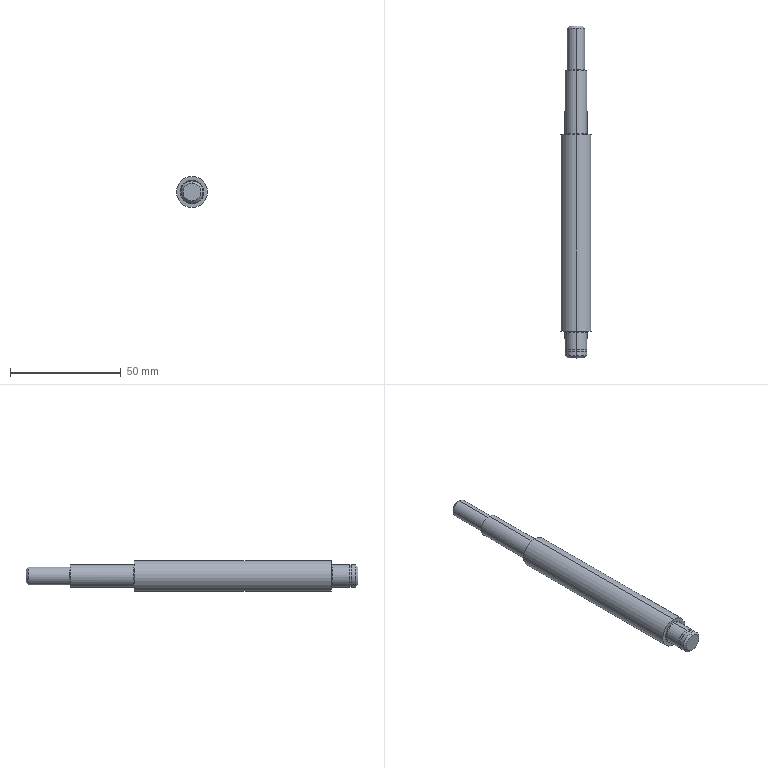Part | SolidWorks | features BaseBody 1 | 1 solid | 29 faces | box 14 x 150 x 14 mm | volume 17893 mm3 | cylinder 12 | plane 7 | spline 6 | cone 4 | commonest cylinder face diameters 10 x6 8 x2 9.6 x2 14 x2
STEP:
#1=CARTESIAN_POINT('',(295.521,1568.164,-1178.061));
#2=VERTEX_POINT('',#1);
#3=CARTESIAN_POINT('',(290.547,1568.164,-1173.57));
#4=VERTEX_POINT('',#3);
#5=CARTESIAN_POINT('',(290.547,1568.164,-1178.57));
#6=DIRECTION('',(0.,-1.,0.));
#7=DIRECTION('',(-0.9948,0.,-0.1018));
#8=AXIS2_PLACEMENT_3D('',#5,#6,#7);
#9=CIRCLE('',#8,5.);
#10=EDGE_CURVE('',#2,#4,#9,.T.);
#11=ORIENTED_EDGE('',*,*,#10,.F.);
#12=CARTESIAN_POINT('',(295.819,1568.464,-1178.031));
#13=VERTEX_POINT('',#12);
#14=CARTESIAN_POINT('',(295.819,1568.164,-1178.031));
#15=DIRECTION('',(0.1018,0.,-0.9948));
#16=DIRECTION('',(0.9948,0.,0.1018));
#17=AXIS2_PLACEMENT_3D('',#14,#15,#16);
#18=CIRCLE('',#17,0.3);
#19=EDGE_CURVE('',#2,#13,#18,.T.);
#20=ORIENTED_EDGE('',*,*,#19,.T.);
#21=CARTESIAN_POINT('',(285.274,1568.464,-1179.109));
#22=VERTEX_POINT('',#21);
#23=CARTESIAN_POINT('',(295.819,1568.464,-1178.031));
#24=CARTESIAN_POINT('',(295.503,1568.464,-1174.942));
#25=CARTESIAN_POINT('',(293.096,1568.464,-1172.982));
#26=CARTESIAN_POINT('',(290.007,1568.464,-1173.298));
#27=CARTESIAN_POINT('',(286.919,1568.464,-1173.613));
#28=CARTESIAN_POINT('',(284.958,1568.464,-1176.021));
#29=CARTESIAN_POINT('',(285.274,1568.464,-1179.109));
#30=(BOUNDED_CURVE()B_SPLINE_CURVE(3,(#23,#24,#25,#26,#27,#28,#29),.UNSPECIFIED.,.F.,.T.)B_SPLINE_CURVE_WITH_KNOTS((4,3,4),(0.,0.5,1.),.UNSPECIFIED.)CURVE()GEOMETRIC_REPRESENTATION_ITEM()RATIONAL_B_SPLINE_CURVE((1.,0.8047,0.8047,1.,0.8047,0.8047,1.))REPRESENTATION_ITEM(''));
#31=EDGE_CURVE('',#13,#22,#30,.T.);
#32=ORIENTED_EDGE('',*,*,#31,.T.);
#33=CARTESIAN_POINT('',(285.572,1568.164,-1179.079));
#34=VERTEX_POINT('',#33);
#35=CARTESIAN_POINT('',(285.274,1568.164,-1179.109));
#36=DIRECTION('',(-0.1018,0.,0.9948));
#37=DIRECTION('',(-0.9948,0.,-0.1018));
#38=AXIS2_PLACEMENT_3D('',#35,#36,#37);
#39=CIRCLE('',#38,0.3);
#40=EDGE_CURVE('',#34,#22,#39,.T.);
#41=ORIENTED_EDGE('',*,*,#40,.F.);
#42=CARTESIAN_POINT('',(290.547,1568.164,-1178.57));
#43=DIRECTION('',(0.,-1.,0.));
#44=DIRECTION('',(-0.9948,0.,-0.1018));
#45=AXIS2_PLACEMENT_3D('',#42,#43,#44);
#46=CIRCLE('',#45,5.);
#47=EDGE_CURVE('',#4,#34,#46,.T.);
#48=ORIENTED_EDGE('',*,*,#47,.F.);
#49=EDGE_LOOP('',(#11,#20,#32,#41,#48));
#50=FACE_OUTER_BOUND('',#49,.T.);
#51=CARTESIAN_POINT('',(285.572,1568.164,-1179.079));
#52=CARTESIAN_POINT('',(285.274,1568.164,-1176.165));
#53=CARTESIAN_POINT('',(287.124,1568.164,-1173.894));
#54=CARTESIAN_POINT('',(290.038,1568.164,-1173.596));
#55=CARTESIAN_POINT('',(292.951,1568.164,-1173.298));
#56=CARTESIAN_POINT('',(295.222,1568.164,-1175.147));
#57=CARTESIAN_POINT('',(295.521,1568.164,-1178.061));
#58=CARTESIAN_POINT('',(285.572,1568.34,-1179.079));
#59=CARTESIAN_POINT('',(285.274,1568.34,-1176.165));
#60=CARTESIAN_POINT('',(287.124,1568.34,-1173.894));
#61=CARTESIAN_POINT('',(290.038,1568.34,-1173.596));
#62=CARTESIAN_POINT('',(292.951,1568.34,-1173.298));
#63=CARTESIAN_POINT('',(295.222,1568.34,-1175.147));
#64=CARTESIAN_POINT('',(295.521,1568.34,-1178.061));
#65=CARTESIAN_POINT('',(285.449,1568.464,-1179.091));
#66=CARTESIAN_POINT('',(285.143,1568.464,-1176.105));
#67=CARTESIAN_POINT('',(287.039,1568.464,-1173.778));
#68=CARTESIAN_POINT('',(290.025,1568.464,-1173.472));
#69=CARTESIAN_POINT('',(293.011,1568.464,-1173.167));
#70=CARTESIAN_POINT('',(295.339,1568.464,-1175.062));
#71=CARTESIAN_POINT('',(295.644,1568.464,-1178.049));
#72=CARTESIAN_POINT('',(285.274,1568.464,-1179.109));
#73=CARTESIAN_POINT('',(284.958,1568.464,-1176.021));
#74=CARTESIAN_POINT('',(286.919,1568.464,-1173.613));
#75=CARTESIAN_POINT('',(290.007,1568.464,-1173.298));
#76=CARTESIAN_POINT('',(293.096,1568.464,-1172.982));
#77=CARTESIAN_POINT('',(295.503,1568.464,-1174.942));
#78=CARTESIAN_POINT('',(295.819,1568.464,-1178.031));
#79=(BOUNDED_SURFACE()B_SPLINE_SURFACE(3,3,((#51,#52,#53,#54,#55,#56,#57),(#58,#59,#60,#61,#62,#63,#64),(#65,#66,#67,#68,#69,#70,#71),(#72,#73,#74,#75,#76,#77,#78)),.UNSPECIFIED.,.F.,.F.,.F.)B_SPLINE_SURFACE_WITH_KNOTS((4,4),(4,3,4),(0.,1.),(0.,0.5,1.),.UNSPECIFIED.)GEOMETRIC_REPRESENTATION_ITEM()RATIONAL_B_SPLINE_SURFACE(((1.,0.8047,0.8047,1.,0.8047,0.8047,1.),(0.8047,0.6476,0.6476,0.8047,0.6476,0.6476,0.8047),(0.8047,0.6476,0.6476,0.8047,0.6476,0.6476,0.8047),(1.,0.8047,0.8047,1.,0.8047,0.8047,1.)))REPRESENTATION_ITEM('')SURFACE());
#80=ADVANCED_FACE('',(#50),#79,.F.);
#81=CARTESIAN_POINT('',(285.572,1657.764,-1179.079));
#82=VERTEX_POINT('',#81);
#83=CARTESIAN_POINT('',(290.547,1657.764,-1173.57));
#84=VERTEX_POINT('',#83);
#85=CARTESIAN_POINT('',(290.547,1657.764,-1178.57));
#86=DIRECTION('',(0.,1.,0.));
#87=DIRECTION('',(0.9948,0.,0.1018));
#88=AXIS2_PLACEMENT_3D('',#85,#86,#87);
#89=CIRCLE('',#88,5.);
#90=EDGE_CURVE('',#82,#84,#89,.T.);
#91=ORIENTED_EDGE('',*,*,#90,.F.);
#92=CARTESIAN_POINT('',(285.274,1657.464,-1179.109));
#93=VERTEX_POINT('',#92);
#94=CARTESIAN_POINT('',(285.274,1657.764,-1179.109));
#95=DIRECTION('',(0.1018,0.,-0.9948));
#96=DIRECTION('',(-0.9948,0.,-0.1018));
#97=AXIS2_PLACEMENT_3D('',#94,#95,#96);
#98=CIRCLE('',#97,0.3);
#99=EDGE_CURVE('',#82,#93,#98,.T.);
#100=ORIENTED_EDGE('',*,*,#99,.T.);
#101=CARTESIAN_POINT('',(295.819,1657.464,-1178.031));
#102=VERTEX_POINT('',#101);
#103=CARTESIAN_POINT('',(285.274,1657.464,-1179.109));
#104=CARTESIAN_POINT('',(284.958,1657.464,-1176.021));
#105=CARTESIAN_POINT('',(286.919,1657.464,-1173.613));
#106=CARTESIAN_POINT('',(290.007,1657.464,-1173.298));
#107=CARTESIAN_POINT('',(293.096,1657.464,-1172.982));
#108=CARTESIAN_POINT('',(295.503,1657.464,-1174.942));
#109=CARTESIAN_POINT('',(295.819,1657.464,-1178.031));
#110=(BOUNDED_CURVE()B_SPLINE_CURVE(3,(#103,#104,#105,#106,#107,#108,#109),.UNSPECIFIED.,.F.,.T.)B_SPLINE_CURVE_WITH_KNOTS((4,3,4),(0.,0.5,1.),.UNSPECIFIED.)CURVE()GEOMETRIC_REPRESENTATION_ITEM()RATIONAL_B_SPLINE_CURVE((1.,0.8047,0.8047,1.,0.8047,0.8047,1.))REPRESENTATION_ITEM(''));
#111=EDGE_CURVE('',#93,#102,#110,.T.);
#112=ORIENTED_EDGE('',*,*,#111,.T.);
#113=CARTESIAN_POINT('',(295.521,1657.764,-1178.061));
#114=VERTEX_POINT('',#113);
#115=CARTESIAN_POINT('',(295.819,1657.764,-1178.031));
#116=DIRECTION('',(-0.1018,0.,0.9948));
#117=DIRECTION('',(0.9948,0.,0.1018));
#118=AXIS2_PLACEMENT_3D('',#115,#116,#117);
#119=CIRCLE('',#118,0.3);
#120=EDGE_CURVE('',#114,#102,#119,.T.);
#121=ORIENTED_EDGE('',*,*,#120,.F.);
#122=CARTESIAN_POINT('',(290.547,1657.764,-1178.57));
#123=DIRECTION('',(0.,1.,0.));
#124=DIRECTION('',(0.9948,0.,0.1018));
#125=AXIS2_PLACEMENT_3D('',#122,#123,#124);
#126=CIRCLE('',#125,5.);
#127=EDGE_CURVE('',#84,#114,#126,.T.);
#128=ORIENTED_EDGE('',*,*,#127,.F.);
#129=EDGE_LOOP('',(#91,#100,#112,#121,#128));
#130=FACE_OUTER_BOUND('',#129,.T.);
#131=CARTESIAN_POINT('',(295.521,1657.764,-1178.061));
#132=CARTESIAN_POINT('',(295.222,1657.764,-1175.147));
#133=CARTESIAN_POINT('',(292.951,1657.764,-1173.298));
#134=CARTESIAN_POINT('',(290.038,1657.764,-1173.596));
#135=CARTESIAN_POINT('',(287.124,1657.764,-1173.894));
#136=CARTESIAN_POINT('',(285.274,1657.764,-1176.165));
#137=CARTESIAN_POINT('',(285.572,1657.764,-1179.079));
#138=CARTESIAN_POINT('',(295.521,1657.588,-1178.061));
#139=CARTESIAN_POINT('',(295.222,1657.588,-1175.147));
#140=CARTESIAN_POINT('',(292.951,1657.588,-1173.298));
#141=CARTESIAN_POINT('',(290.038,1657.588,-1173.596));
#142=CARTESIAN_POINT('',(287.124,1657.588,-1173.894));
#143=CARTESIAN_POINT('',(285.274,1657.588,-1176.165));
#144=CARTESIAN_POINT('',(285.572,1657.588,-1179.079));
#145=CARTESIAN_POINT('',(295.644,1657.464,-1178.049));
#146=CARTESIAN_POINT('',(295.339,1657.464,-1175.062));
#147=CARTESIAN_POINT('',(293.011,1657.464,-1173.167));
#148=CARTESIAN_POINT('',(290.025,1657.464,-1173.472));
#149=CARTESIAN_POINT('',(287.039,1657.464,-1173.778));
#150=CARTESIAN_POINT('',(285.143,1657.464,-1176.105));
#151=CARTESIAN_POINT('',(285.449,1657.464,-1179.091));
#152=CARTESIAN_POINT('',(295.819,1657.464,-1178.031));
#153=CARTESIAN_POINT('',(295.503,1657.464,-1174.942));
#154=CARTESIAN_POINT('',(293.096,1657.464,-1172.982));
#155=CARTESIAN_POINT('',(290.007,1657.464,-1173.298));
#156=CARTESIAN_POINT('',(286.919,1657.464,-1173.613));
#157=CARTESIAN_POINT('',(284.958,1657.464,-1176.021));
#158=CARTESIAN_POINT('',(285.274,1657.464,-1179.109));
#159=(BOUNDED_SURFACE()B_SPLINE_SURFACE(3,3,((#131,#132,#133,#134,#135,#136,#137),(#138,#139,#140,#141,#142,#143,#144),(#145,#146,#147,#148,#149,#150,#151),(#152,#153,#154,#155,#156,#157,#158)),.UNSPECIFIED.,.F.,.F.,.F.)B_SPLINE_SURFACE_WITH_KNOTS((4,4),(4,3,4),(0.,1.),(0.,0.5,1.),.UNSPECIFIED.)GEOMETRIC_REPRESENTATION_ITEM()RATIONAL_B_SPLINE_SURFACE(((1.,0.8047,0.8047,1.,0.8047,0.8047,1.),(0.8047,0.6476,0.6476,0.8047,0.6476,0.6476,0.8047),(0.8047,0.6476,0.6476,0.8047,0.6476,0.6476,0.8047),(1.,0.8047,0.8047,1.,0.8047,0.8047,1.)))REPRESENTATION_ITEM('')SURFACE());
#160=ADVANCED_FACE('',(#130),#159,.F.);
#161=CARTESIAN_POINT('',(286.567,1686.764,-1178.977));
#162=VERTEX_POINT('',#161);
#163=CARTESIAN_POINT('',(290.547,1686.764,-1174.57));
#164=VERTEX_POINT('',#163);
#165=CARTESIAN_POINT('',(290.547,1686.764,-1178.57));
#166=DIRECTION('',(0.,1.,0.));
#167=DIRECTION('',(0.9948,0.,0.1018));
#168=AXIS2_PLACEMENT_3D('',#165,#166,#167);
#169=CIRCLE('',#168,4.);
#170=EDGE_CURVE('',#162,#164,#169,.T.);
#171=ORIENTED_EDGE('',*,*,#170,.F.);
#172=CARTESIAN_POINT('',(286.269,1686.464,-1179.008));
#173=VERTEX_POINT('',#172);
#174=CARTESIAN_POINT('',(286.269,1686.764,-1179.008));
#175=DIRECTION('',(0.1018,0.,-0.9948));
#176=DIRECTION('',(-0.9948,0.,-0.1018));
#177=AXIS2_PLACEMENT_3D('',#174,#175,#176);
#178=CIRCLE('',#177,0.3);
#179=EDGE_CURVE('',#162,#173,#178,.T.);
#180=ORIENTED_EDGE('',*,*,#179,.T.);
#181=CARTESIAN_POINT('',(294.824,1686.464,-1178.132));
#182=VERTEX_POINT('',#181);
#183=CARTESIAN_POINT('',(286.269,1686.464,-1179.008));
#184=CARTESIAN_POINT('',(285.394,1686.464,-1170.452));
#185=CARTESIAN_POINT('',(293.949,1686.464,-1169.577));
#186=CARTESIAN_POINT('',(294.824,1686.464,-1178.132));
#187=(BOUNDED_CURVE()B_SPLINE_CURVE(3,(#183,#184,#185,#186),.UNSPECIFIED.,.F.,.T.)B_SPLINE_CURVE_WITH_KNOTS((4,4),(0.,1.),.UNSPECIFIED.)CURVE()GEOMETRIC_REPRESENTATION_ITEM()RATIONAL_B_SPLINE_CURVE((1.,0.3333,0.3333,1.))REPRESENTATION_ITEM(''));
#188=EDGE_CURVE('',#173,#182,#187,.T.);
#189=ORIENTED_EDGE('',*,*,#188,.T.);
#190=CARTESIAN_POINT('',(294.526,1686.764,-1178.163));
#191=VERTEX_POINT('',#190);
#192=CARTESIAN_POINT('',(294.824,1686.764,-1178.132));
#193=DIRECTION('',(-0.1018,0.,0.9948));
#194=DIRECTION('',(0.9948,0.,0.1018));
#195=AXIS2_PLACEMENT_3D('',#192,#193,#194);
#196=CIRCLE('',#195,0.3);
#197=EDGE_CURVE('',#191,#182,#196,.T.);
#198=ORIENTED_EDGE('',*,*,#197,.F.);
#199=CARTESIAN_POINT('',(290.547,1686.764,-1178.57));
#200=DIRECTION('',(0.,1.,0.));
#201=DIRECTION('',(0.9948,0.,0.1018));
#202=AXIS2_PLACEMENT_3D('',#199,#200,#201);
#203=CIRCLE('',#202,4.);
#204=EDGE_CURVE('',#164,#191,#203,.T.);
#205=ORIENTED_EDGE('',*,*,#204,.F.);
#206=EDGE_LOOP('',(#171,#180,#189,#198,#205));
#207=FACE_OUTER_BOUND('',#206,.T.);
#208=CARTESIAN_POINT('',(294.526,1686.764,-1178.163));
#209=CARTESIAN_POINT('',(293.712,1686.764,-1170.204));
#210=CARTESIAN_POINT('',(285.753,1686.764,-1171.019));
#211=CARTESIAN_POINT('',(286.567,1686.764,-1178.977));
#212=CARTESIAN_POINT('',(294.526,1686.588,-1178.163));
#213=CARTESIAN_POINT('',(293.712,1686.588,-1170.204));
#214=CARTESIAN_POINT('',(285.753,1686.588,-1171.019));
#215=CARTESIAN_POINT('',(286.567,1686.588,-1178.977));
#216=CARTESIAN_POINT('',(294.649,1686.464,-1178.15));
#217=CARTESIAN_POINT('',(293.81,1686.464,-1169.945));
#218=CARTESIAN_POINT('',(285.604,1686.464,-1170.784));
#219=CARTESIAN_POINT('',(286.444,1686.464,-1178.99));
#220=CARTESIAN_POINT('',(294.824,1686.464,-1178.132));
#221=CARTESIAN_POINT('',(293.949,1686.464,-1169.577));
#222=CARTESIAN_POINT('',(285.394,1686.464,-1170.452));
#223=CARTESIAN_POINT('',(286.269,1686.464,-1179.008));
#224=(BOUNDED_SURFACE()B_SPLINE_SURFACE(3,3,((#208,#209,#210,#211),(#212,#213,#214,#215),(#216,#217,#218,#219),(#220,#221,#222,#223)),.UNSPECIFIED.,.F.,.F.,.F.)B_SPLINE_SURFACE_WITH_KNOTS((4,4),(4,4),(0.,1.),(0.,1.),.UNSPECIFIED.)GEOMETRIC_REPRESENTATION_ITEM()RATIONAL_B_SPLINE_SURFACE(((1.,0.3333,0.3333,1.),(0.8047,0.2682,0.2682,0.8047),(0.8047,0.2682,0.2682,0.8047),(1.,0.3333,0.3333,1.)))REPRESENTATION_ITEM('')SURFACE());
#225=ADVANCED_FACE('',(#207),#224,.F.);
#226=CARTESIAN_POINT('',(290.547,1657.464,-1185.57));
#227=VERTEX_POINT('',#226);
#228=CARTESIAN_POINT('',(290.547,1657.464,-1171.57));
#229=VERTEX_POINT('',#228);
#230=CARTESIAN_POINT('',(290.547,1657.464,-1178.57));
#231=DIRECTION('',(0.,-1.,0.));
#232=DIRECTION('',(0.,0.,-1.));
#233=AXIS2_PLACEMENT_3D('',#230,#231,#232);
#234=CIRCLE('',#233,7.);
#235=EDGE_CURVE('',#227,#229,#234,.T.);
#236=ORIENTED_EDGE('',*,*,#235,.T.);
#237=CARTESIAN_POINT('',(290.547,1568.464,-1171.57));
#238=VERTEX_POINT('',#237);
#239=CARTESIAN_POINT('',(290.547,1556.464,-1171.57));
#240=DIRECTION('',(0.,-1.,0.));
#241=VECTOR('',#240,1000.);
#242=LINE('',#239,#241);
#243=EDGE_CURVE('',#229,#238,#242,.T.);
#244=ORIENTED_EDGE('',*,*,#243,.T.);
#245=CARTESIAN_POINT('',(290.547,1568.464,-1185.57));
#246=VERTEX_POINT('',#245);
#247=CARTESIAN_POINT('',(290.547,1568.464,-1178.57));
#248=DIRECTION('',(0.,1.,0.));
#249=DIRECTION('',(0.,0.,-1.));
#250=AXIS2_PLACEMENT_3D('',#247,#248,#249);
#251=CIRCLE('',#250,7.);
#252=EDGE_CURVE('',#238,#246,#251,.T.);
#253=ORIENTED_EDGE('',*,*,#252,.T.);
#254=CARTESIAN_POINT('',(290.547,1556.464,-1185.57));
#255=DIRECTION('',(0.,-1.,0.));
#256=VECTOR('',#255,1000.);
#257=LINE('',#254,#256);
#258=EDGE_CURVE('',#227,#246,#257,.T.);
#259=ORIENTED_EDGE('',*,*,#258,.F.);
#260=EDGE_LOOP('',(#236,#244,#253,#259));
#261=FACE_OUTER_BOUND('',#260,.T.);
#262=CARTESIAN_POINT('',(290.547,1556.464,-1178.57));
#263=DIRECTION('',(0.,-1.,0.));
#264=DIRECTION('',(0.,0.,-1.));
#265=AXIS2_PLACEMENT_3D('',#262,#263,#264);
#266=CYLINDRICAL_SURFACE('',#265,7.);
#267=ADVANCED_FACE('',(#261),#266,.T.);
#268=CARTESIAN_POINT('',(290.547,1568.164,-1183.57));
#269=VERTEX_POINT('',#268);
#270=CARTESIAN_POINT('',(290.547,1568.164,-1178.57));
#271=DIRECTION('',(0.,-1.,0.));
#272=DIRECTION('',(-0.9948,0.,-0.1018));
#273=AXIS2_PLACEMENT_3D('',#270,#271,#272);
#274=CIRCLE('',#273,5.);
#275=EDGE_CURVE('',#269,#2,#274,.T.);
#276=ORIENTED_EDGE('',*,*,#275,.T.);
#277=ORIENTED_EDGE('',*,*,#10,.T.);
#278=CARTESIAN_POINT('',(290.547,1560.464,-1173.57));
#279=VERTEX_POINT('',#278);
#280=CARTESIAN_POINT('',(290.547,1556.464,-1173.57));
#281=DIRECTION('',(0.,-1.,0.));
#282=VECTOR('',#281,1000.);
#283=LINE('',#280,#282);
#284=EDGE_CURVE('',#4,#279,#283,.T.);
#285=ORIENTED_EDGE('',*,*,#284,.T.);
#286=CARTESIAN_POINT('',(290.547,1560.464,-1183.57));
#287=VERTEX_POINT('',#286);
#288=CARTESIAN_POINT('',(290.547,1560.464,-1178.57));
#289=DIRECTION('',(0.,1.,0.));
#290=DIRECTION('',(0.,0.,-1.));
#291=AXIS2_PLACEMENT_3D('',#288,#289,#290);
#292=CIRCLE('',#291,5.);
#293=EDGE_CURVE('',#279,#287,#292,.T.);
#294=ORIENTED_EDGE('',*,*,#293,.T.);
#295=CARTESIAN_POINT('',(290.547,1556.464,-1183.57));
#296=DIRECTION('',(0.,-1.,0.));
#297=VECTOR('',#296,1000.);
#298=LINE('',#295,#297);
#299=EDGE_CURVE('',#269,#287,#298,.T.);
#300=ORIENTED_EDGE('',*,*,#299,.F.);
#301=EDGE_LOOP('',(#276,#277,#285,#294,#300));
#302=FACE_OUTER_BOUND('',#301,.T.);
#303=CARTESIAN_POINT('',(290.547,1556.464,-1178.57));
#304=DIRECTION('',(0.,-1.,0.));
#305=DIRECTION('',(0.,0.,-1.));
#306=AXIS2_PLACEMENT_3D('',#303,#304,#305);
#307=CYLINDRICAL_SURFACE('',#306,5.);
#308=ADVANCED_FACE('',(#302),#307,.T.);
#309=CARTESIAN_POINT('',(290.547,1686.464,-1183.57));
#310=VERTEX_POINT('',#309);
#311=CARTESIAN_POINT('',(290.547,1686.464,-1173.57));
#312=VERTEX_POINT('',#311);
#313=CARTESIAN_POINT('',(290.547,1686.464,-1178.57));
#314=DIRECTION('',(0.,-1.,0.));
#315=DIRECTION('',(0.,0.,-1.));
#316=AXIS2_PLACEMENT_3D('',#313,#314,#315);
#317=CIRCLE('',#316,5.);
#318=EDGE_CURVE('',#310,#312,#317,.T.);
#319=ORIENTED_EDGE('',*,*,#318,.T.);
#320=CARTESIAN_POINT('',(290.547,1556.464,-1173.57));
#321=DIRECTION('',(0.,-1.,0.));
#322=VECTOR('',#321,1000.);
#323=LINE('',#320,#322);
#324=EDGE_CURVE('',#312,#84,#323,.T.);
#325=ORIENTED_EDGE('',*,*,#324,.T.);
#326=ORIENTED_EDGE('',*,*,#127,.T.);
#327=CARTESIAN_POINT('',(290.547,1657.764,-1183.57));
#328=VERTEX_POINT('',#327);
#329=CARTESIAN_POINT('',(290.547,1657.764,-1178.57));
#330=DIRECTION('',(0.,1.,0.));
#331=DIRECTION('',(0.9948,0.,0.1018));
#332=AXIS2_PLACEMENT_3D('',#329,#330,#331);
#333=CIRCLE('',#332,5.);
#334=EDGE_CURVE('',#114,#328,#333,.T.);
#335=ORIENTED_EDGE('',*,*,#334,.T.);
#336=CARTESIAN_POINT('',(290.547,1556.464,-1183.57));
#337=DIRECTION('',(0.,-1.,0.));
#338=VECTOR('',#337,1000.);
#339=LINE('',#336,#338);
#340=EDGE_CURVE('',#310,#328,#339,.T.);
#341=ORIENTED_EDGE('',*,*,#340,.F.);
#342=EDGE_LOOP('',(#319,#325,#326,#335,#341));
#343=FACE_OUTER_BOUND('',#342,.T.);
#344=CARTESIAN_POINT('',(290.547,1556.464,-1178.57));
#345=DIRECTION('',(0.,-1.,0.));
#346=DIRECTION('',(0.,0.,-1.));
#347=AXIS2_PLACEMENT_3D('',#344,#345,#346);
#348=CYLINDRICAL_SURFACE('',#347,5.);
#349=ADVANCED_FACE('',(#343),#348,.T.);
#350=CARTESIAN_POINT('',(290.547,1560.464,-1183.37));
#351=VERTEX_POINT('',#350);
#352=CARTESIAN_POINT('',(290.547,1560.464,-1173.77));
#353=VERTEX_POINT('',#352);
#354=CARTESIAN_POINT('',(290.547,1560.464,-1178.57));
#355=DIRECTION('',(0.,-1.,0.));
#356=DIRECTION('',(0.,0.,-1.));
#357=AXIS2_PLACEMENT_3D('',#354,#355,#356);
#358=CIRCLE('',#357,4.8);
#359=EDGE_CURVE('',#351,#353,#358,.T.);
#360=ORIENTED_EDGE('',*,*,#359,.T.);
#361=CARTESIAN_POINT('',(290.547,1559.314,-1173.77));
#362=VERTEX_POINT('',#361);
#363=CARTESIAN_POINT('',(290.547,1556.464,-1173.77));
#364=DIRECTION('',(0.,-1.,0.));
#365=VECTOR('',#364,1000.);
#366=LINE('',#363,#365);
#367=EDGE_CURVE('',#353,#362,#366,.T.);
#368=ORIENTED_EDGE('',*,*,#367,.T.);
#369=CARTESIAN_POINT('',(290.547,1559.314,-1183.37));
#370=VERTEX_POINT('',#369);
#371=CARTESIAN_POINT('',(290.547,1559.314,-1178.57));
#372=DIRECTION('',(0.,1.,0.));
#373=DIRECTION('',(0.,0.,-1.));
#374=AXIS2_PLACEMENT_3D('',#371,#372,#373);
#375=CIRCLE('',#374,4.8);
#376=EDGE_CURVE('',#362,#370,#375,.T.);
#377=ORIENTED_EDGE('',*,*,#376,.T.);
#378=CARTESIAN_POINT('',(290.547,1556.464,-1183.37));
#379=DIRECTION('',(0.,-1.,0.));
#380=VECTOR('',#379,1000.);
#381=LINE('',#378,#380);
#382=EDGE_CURVE('',#351,#370,#381,.T.);
#383=ORIENTED_EDGE('',*,*,#382,.F.);
#384=EDGE_LOOP('',(#360,#368,#377,#383));
#385=FACE_OUTER_BOUND('',#384,.T.);
#386=CARTESIAN_POINT('',(290.547,1556.464,-1178.57));
#387=DIRECTION('',(0.,-1.,0.));
#388=DIRECTION('',(0.,0.,-1.));
#389=AXIS2_PLACEMENT_3D('',#386,#387,#388);
#390=CYLINDRICAL_SURFACE('',#389,4.8);
#391=ADVANCED_FACE('',(#385),#390,.T.);
#392=CARTESIAN_POINT('',(290.547,1559.314,-1183.57));
#393=VERTEX_POINT('',#392);
#394=CARTESIAN_POINT('',(290.547,1559.314,-1173.57));
#395=VERTEX_POINT('',#394);
#396=CARTESIAN_POINT('',(290.547,1559.314,-1178.57));
#397=DIRECTION('',(0.,-1.,0.));
#398=DIRECTION('',(0.,0.,-1.));
#399=AXIS2_PLACEMENT_3D('',#396,#397,#398);
#400=CIRCLE('',#399,5.);
#401=EDGE_CURVE('',#393,#395,#400,.T.);
#402=ORIENTED_EDGE('',*,*,#401,.T.);
#403=CARTESIAN_POINT('',(290.547,1557.464,-1173.57));
#404=VERTEX_POINT('',#403);
#405=CARTESIAN_POINT('',(290.547,1556.464,-1173.57));
#406=DIRECTION('',(0.,-1.,0.));
#407=VECTOR('',#406,1000.);
#408=LINE('',#405,#407);
#409=EDGE_CURVE('',#395,#404,#408,.T.);
#410=ORIENTED_EDGE('',*,*,#409,.T.);
#411=CARTESIAN_POINT('',(290.547,1557.464,-1183.57));
#412=VERTEX_POINT('',#411);
#413=CARTESIAN_POINT('',(290.547,1557.464,-1178.57));
#414=DIRECTION('',(0.,1.,0.));
#415=DIRECTION('',(0.,0.,-1.));
#416=AXIS2_PLACEMENT_3D('',#413,#414,#415);
#417=CIRCLE('',#416,5.);
#418=EDGE_CURVE('',#404,#412,#417,.T.);
#419=ORIENTED_EDGE('',*,*,#418,.T.);
#420=CARTESIAN_POINT('',(290.547,1556.464,-1183.57));
#421=DIRECTION('',(0.,-1.,0.));
#422=VECTOR('',#421,1000.);
#423=LINE('',#420,#422);
#424=EDGE_CURVE('',#393,#412,#423,.T.);
#425=ORIENTED_EDGE('',*,*,#424,.F.);
#426=EDGE_LOOP('',(#402,#410,#419,#425));
#427=FACE_OUTER_BOUND('',#426,.T.);
#428=CARTESIAN_POINT('',(290.547,1556.464,-1178.57));
#429=DIRECTION('',(0.,-1.,0.));
#430=DIRECTION('',(0.,0.,-1.));
#431=AXIS2_PLACEMENT_3D('',#428,#429,#430);
#432=CYLINDRICAL_SURFACE('',#431,5.);
#433=ADVANCED_FACE('',(#427),#432,.T.);
#434=CARTESIAN_POINT('',(290.547,1705.464,-1182.57));
#435=VERTEX_POINT('',#434);
#436=CARTESIAN_POINT('',(290.547,1705.464,-1174.57));
#437=VERTEX_POINT('',#436);
#438=CARTESIAN_POINT('',(290.547,1705.464,-1178.57));
#439=DIRECTION('',(0.,-1.,0.));
#440=DIRECTION('',(0.,0.,-1.));
#441=AXIS2_PLACEMENT_3D('',#438,#439,#440);
#442=CIRCLE('',#441,4.);
#443=EDGE_CURVE('',#435,#437,#442,.T.);
#444=ORIENTED_EDGE('',*,*,#443,.T.);
#445=CARTESIAN_POINT('',(290.547,1556.464,-1174.57));
#446=DIRECTION('',(0.,-1.,0.));
#447=VECTOR('',#446,1000.);
#448=LINE('',#445,#447);
#449=EDGE_CURVE('',#437,#164,#448,.T.);
#450=ORIENTED_EDGE('',*,*,#449,.T.);
#451=ORIENTED_EDGE('',*,*,#204,.T.);
#452=CARTESIAN_POINT('',(290.547,1686.764,-1182.57));
#453=VERTEX_POINT('',#452);
#454=CARTESIAN_POINT('',(290.547,1686.764,-1178.57));
#455=DIRECTION('',(0.,1.,0.));
#456=DIRECTION('',(0.9948,0.,0.1018));
#457=AXIS2_PLACEMENT_3D('',#454,#455,#456);
#458=CIRCLE('',#457,4.);
#459=EDGE_CURVE('',#191,#453,#458,.T.);
#460=ORIENTED_EDGE('',*,*,#459,.T.);
#461=CARTESIAN_POINT('',(290.547,1556.464,-1182.57));
#462=DIRECTION('',(0.,-1.,0.));
#463=VECTOR('',#462,1000.);
#464=LINE('',#461,#463);
#465=EDGE_CURVE('',#435,#453,#464,.T.);
#466=ORIENTED_EDGE('',*,*,#465,.F.);
#467=EDGE_LOOP('',(#444,#450,#451,#460,#466));
#468=FACE_OUTER_BOUND('',#467,.T.);
#469=CARTESIAN_POINT('',(290.547,1556.464,-1178.57));
#470=DIRECTION('',(0.,-1.,0.));
#471=DIRECTION('',(0.,0.,-1.));
#472=AXIS2_PLACEMENT_3D('',#469,#470,#471);
#473=CYLINDRICAL_SURFACE('',#472,4.);
#474=ADVANCED_FACE('',(#468),#473,.T.);
#475=CARTESIAN_POINT('',(290.547,1556.464,-1174.57));
#476=VERTEX_POINT('',#475);
#477=CARTESIAN_POINT('',(290.547,1556.464,-1182.57));
#478=VERTEX_POINT('',#477);
#479=CARTESIAN_POINT('',(290.547,1556.464,-1178.57));
#480=DIRECTION('',(0.,1.,0.));
#481=DIRECTION('',(0.,0.,1.));
#482=AXIS2_PLACEMENT_3D('',#479,#480,#481);
#483=CIRCLE('',#482,4.);
#484=EDGE_CURVE('',#476,#478,#483,.T.);
#485=ORIENTED_EDGE('',*,*,#484,.T.);
#486=CARTESIAN_POINT('',(290.547,1557.464,-1183.57));
#487=DIRECTION('',(0.,0.7071,-0.7071));
#488=VECTOR('',#487,1000.);
#489=LINE('',#486,#488);
#490=EDGE_CURVE('',#478,#412,#489,.T.);
#491=ORIENTED_EDGE('',*,*,#490,.T.);
#492=ORIENTED_EDGE('',*,*,#418,.F.);
#493=CARTESIAN_POINT('',(290.547,1557.464,-1173.57));
#494=DIRECTION('',(0.,0.7071,0.7071));
#495=VECTOR('',#494,1000.);
#496=LINE('',#493,#495);
#497=EDGE_CURVE('',#476,#404,#496,.T.);
#498=ORIENTED_EDGE('',*,*,#497,.F.);
#499=EDGE_LOOP('',(#485,#491,#492,#498));
#500=FACE_OUTER_BOUND('',#499,.T.);
#501=CARTESIAN_POINT('',(290.547,1557.464,-1178.57));
#502=DIRECTION('',(0.,1.,0.));
#503=DIRECTION('',(0.,0.,1.));
#504=AXIS2_PLACEMENT_3D('',#501,#502,#503);
#505=CONICAL_SURFACE('',#504,5.,0.7854);
#506=ADVANCED_FACE('',(#500),#505,.T.);
#507=CARTESIAN_POINT('',(290.547,1706.464,-1181.57));
#508=VERTEX_POINT('',#507);
#509=CARTESIAN_POINT('',(290.547,1706.464,-1175.57));
#510=VERTEX_POINT('',#509);
#511=CARTESIAN_POINT('',(290.547,1706.464,-1178.57));
#512=DIRECTION('',(0.,-1.,0.));
#513=DIRECTION('',(0.,0.,-1.));
#514=AXIS2_PLACEMENT_3D('',#511,#512,#513);
#515=CIRCLE('',#514,3.);
#516=EDGE_CURVE('',#508,#510,#515,.T.);
#517=ORIENTED_EDGE('',*,*,#516,.T.);
#518=CARTESIAN_POINT('',(290.547,1705.464,-1174.57));
#519=DIRECTION('',(0.,-0.7071,0.7071));
#520=VECTOR('',#519,1000.);
#521=LINE('',#518,#520);
#522=EDGE_CURVE('',#510,#437,#521,.T.);
#523=ORIENTED_EDGE('',*,*,#522,.T.);
#524=ORIENTED_EDGE('',*,*,#443,.F.);
#525=CARTESIAN_POINT('',(290.547,1705.464,-1182.57));
#526=DIRECTION('',(0.,-0.7071,-0.7071));
#527=VECTOR('',#526,1000.);
#528=LINE('',#525,#527);
#529=EDGE_CURVE('',#508,#435,#528,.T.);
#530=ORIENTED_EDGE('',*,*,#529,.F.);
#531=EDGE_LOOP('',(#517,#523,#524,#530));
#532=FACE_OUTER_BOUND('',#531,.T.);
#533=CARTESIAN_POINT('',(290.547,1705.464,-1178.57));
#534=DIRECTION('',(0.,-1.,0.));
#535=DIRECTION('',(0.,0.,-1.));
#536=AXIS2_PLACEMENT_3D('',#533,#534,#535);
#537=CONICAL_SURFACE('',#536,4.,0.7854);
#538=ADVANCED_FACE('',(#532),#537,.T.);
#539=ORIENTED_EDGE('',*,*,#243,.F.);
#540=CARTESIAN_POINT('',(290.547,1657.464,-1178.57));
#541=DIRECTION('',(0.,-1.,0.));
#542=DIRECTION('',(0.,0.,-1.));
#543=AXIS2_PLACEMENT_3D('',#540,#541,#542);
#544=CIRCLE('',#543,7.);
#545=EDGE_CURVE('',#229,#227,#544,.T.);
#546=ORIENTED_EDGE('',*,*,#545,.T.);
#547=ORIENTED_EDGE('',*,*,#258,.T.);
#548=CARTESIAN_POINT('',(290.547,1568.464,-1178.57));
#549=DIRECTION('',(0.,1.,0.));
#550=DIRECTION('',(0.,0.,-1.));
#551=AXIS2_PLACEMENT_3D('',#548,#549,#550);
#552=CIRCLE('',#551,7.);
#553=EDGE_CURVE('',#246,#238,#552,.T.);
#554=ORIENTED_EDGE('',*,*,#553,.T.);
#555=EDGE_LOOP('',(#539,#546,#547,#554));
#556=FACE_OUTER_BOUND('',#555,.T.);
#557=CARTESIAN_POINT('',(290.547,1556.464,-1178.57));
#558=DIRECTION('',(0.,-1.,0.));
#559=DIRECTION('',(0.,0.,-1.));
#560=AXIS2_PLACEMENT_3D('',#557,#558,#559);
#561=CYLINDRICAL_SURFACE('',#560,7.);
#562=ADVANCED_FACE('',(#556),#561,.T.);
#563=ORIENTED_EDGE('',*,*,#31,.F.);
#564=CARTESIAN_POINT('',(285.274,1568.464,-1179.109));
#565=CARTESIAN_POINT('',(285.59,1568.464,-1182.198));
#566=CARTESIAN_POINT('',(287.997,1568.464,-1184.158));
#567=CARTESIAN_POINT('',(291.086,1568.464,-1183.842));
#568=CARTESIAN_POINT('',(294.174,1568.464,-1183.527));
#569=CARTESIAN_POINT('',(296.135,1568.464,-1181.119));
#570=CARTESIAN_POINT('',(295.819,1568.464,-1178.031));
#571=(BOUNDED_CURVE()B_SPLINE_CURVE(3,(#564,#565,#566,#567,#568,#569,#570),.UNSPECIFIED.,.F.,.T.)B_SPLINE_CURVE_WITH_KNOTS((4,3,4),(0.,0.5,1.),.UNSPECIFIED.)CURVE()GEOMETRIC_REPRESENTATION_ITEM()RATIONAL_B_SPLINE_CURVE((1.,0.8047,0.8047,1.,0.8047,0.8047,1.))REPRESENTATION_ITEM(''));
#572=EDGE_CURVE('',#22,#13,#571,.T.);
#573=ORIENTED_EDGE('',*,*,#572,.F.);
#574=EDGE_LOOP('',(#563,#573));
#575=FACE_BOUND('',#574,.T.);
#576=ORIENTED_EDGE('',*,*,#553,.F.);
#577=ORIENTED_EDGE('',*,*,#252,.F.);
#578=EDGE_LOOP('',(#576,#577));
#579=FACE_OUTER_BOUND('',#578,.T.);
#580=CARTESIAN_POINT('',(285.572,1568.464,-1179.079));
#581=DIRECTION('',(0.,1.,0.));
#582=DIRECTION('',(0.,0.,1.));
#583=AXIS2_PLACEMENT_3D('',#580,#581,#582);
#584=PLANE('',#583);
#585=ADVANCED_FACE('',(#575,#579),#584,.F.);
#586=ORIENTED_EDGE('',*,*,#111,.F.);
#587=CARTESIAN_POINT('',(295.819,1657.464,-1178.031));
#588=CARTESIAN_POINT('',(296.898,1657.464,-1188.576));
#589=CARTESIAN_POINT('',(286.353,1657.464,-1189.654));
#590=CARTESIAN_POINT('',(285.274,1657.464,-1179.109));
#591=(BOUNDED_CURVE()B_SPLINE_CURVE(3,(#587,#588,#589,#590),.UNSPECIFIED.,.F.,.T.)B_SPLINE_CURVE_WITH_KNOTS((4,4),(0.,1.),.UNSPECIFIED.)CURVE()GEOMETRIC_REPRESENTATION_ITEM()RATIONAL_B_SPLINE_CURVE((1.,0.3333,0.3333,1.))REPRESENTATION_ITEM(''));
#592=EDGE_CURVE('',#102,#93,#591,.T.);
#593=ORIENTED_EDGE('',*,*,#592,.F.);
#594=EDGE_LOOP('',(#586,#593));
#595=FACE_BOUND('',#594,.T.);
#596=ORIENTED_EDGE('',*,*,#235,.F.);
#597=ORIENTED_EDGE('',*,*,#545,.F.);
#598=EDGE_LOOP('',(#596,#597));
#599=FACE_OUTER_BOUND('',#598,.T.);
#600=CARTESIAN_POINT('',(283.583,1657.464,-1179.282));
#601=DIRECTION('',(0.,-1.,0.));
#602=DIRECTION('',(0.,0.,-1.));
#603=AXIS2_PLACEMENT_3D('',#600,#601,#602);
#604=PLANE('',#603);
#605=ADVANCED_FACE('',(#595,#599),#604,.F.);
#606=ORIENTED_EDGE('',*,*,#19,.F.);
#607=ORIENTED_EDGE('',*,*,#275,.F.);
#608=CARTESIAN_POINT('',(290.547,1568.164,-1178.57));
#609=DIRECTION('',(0.,-1.,0.));
#610=DIRECTION('',(-0.9948,0.,-0.1018));
#611=AXIS2_PLACEMENT_3D('',#608,#609,#610);
#612=CIRCLE('',#611,5.);
#613=EDGE_CURVE('',#34,#269,#612,.T.);
#614=ORIENTED_EDGE('',*,*,#613,.F.);
#615=ORIENTED_EDGE('',*,*,#40,.T.);
#616=ORIENTED_EDGE('',*,*,#572,.T.);
#617=EDGE_LOOP('',(#606,#607,#614,#615,#616));
#618=FACE_OUTER_BOUND('',#617,.T.);
#619=CARTESIAN_POINT('',(295.521,1568.164,-1178.061));
#620=CARTESIAN_POINT('',(295.819,1568.164,-1180.975));
#621=CARTESIAN_POINT('',(293.969,1568.164,-1183.246));
#622=CARTESIAN_POINT('',(291.055,1568.164,-1183.544));
#623=CARTESIAN_POINT('',(288.142,1568.164,-1183.842));
#624=CARTESIAN_POINT('',(285.871,1568.164,-1181.993));
#625=CARTESIAN_POINT('',(285.572,1568.164,-1179.079));
#626=CARTESIAN_POINT('',(295.521,1568.34,-1178.061));
#627=CARTESIAN_POINT('',(295.819,1568.34,-1180.975));
#628=CARTESIAN_POINT('',(293.969,1568.34,-1183.246));
#629=CARTESIAN_POINT('',(291.055,1568.34,-1183.544));
#630=CARTESIAN_POINT('',(288.142,1568.34,-1183.842));
#631=CARTESIAN_POINT('',(285.871,1568.34,-1181.993));
#632=CARTESIAN_POINT('',(285.572,1568.34,-1179.079));
#633=CARTESIAN_POINT('',(295.644,1568.464,-1178.049));
#634=CARTESIAN_POINT('',(295.95,1568.464,-1181.035));
#635=CARTESIAN_POINT('',(294.054,1568.464,-1183.362));
#636=CARTESIAN_POINT('',(291.068,1568.464,-1183.668));
#637=CARTESIAN_POINT('',(288.082,1568.464,-1183.973));
#638=CARTESIAN_POINT('',(285.754,1568.464,-1182.078));
#639=CARTESIAN_POINT('',(285.449,1568.464,-1179.091));
#640=CARTESIAN_POINT('',(295.819,1568.464,-1178.031));
#641=CARTESIAN_POINT('',(296.135,1568.464,-1181.119));
#642=CARTESIAN_POINT('',(294.174,1568.464,-1183.527));
#643=CARTESIAN_POINT('',(291.086,1568.464,-1183.842));
#644=CARTESIAN_POINT('',(287.997,1568.464,-1184.158));
#645=CARTESIAN_POINT('',(285.59,1568.464,-1182.198));
#646=CARTESIAN_POINT('',(285.274,1568.464,-1179.109));
#647=(BOUNDED_SURFACE()B_SPLINE_SURFACE(3,3,((#619,#620,#621,#622,#623,#624,#625),(#626,#627,#628,#629,#630,#631,#632),(#633,#634,#635,#636,#637,#638,#639),(#640,#641,#642,#643,#644,#645,#646)),.UNSPECIFIED.,.F.,.F.,.F.)B_SPLINE_SURFACE_WITH_KNOTS((4,4),(4,3,4),(0.,1.),(0.,0.5,1.),.UNSPECIFIED.)GEOMETRIC_REPRESENTATION_ITEM()RATIONAL_B_SPLINE_SURFACE(((1.,0.8047,0.8047,1.,0.8047,0.8047,1.),(0.8047,0.6476,0.6476,0.8047,0.6476,0.6476,0.8047),(0.8047,0.6476,0.6476,0.8047,0.6476,0.6476,0.8047),(1.,0.8047,0.8047,1.,0.8047,0.8047,1.)))REPRESENTATION_ITEM('')SURFACE());
#648=ADVANCED_FACE('',(#618),#647,.F.);
#649=ORIENTED_EDGE('',*,*,#99,.F.);
#650=CARTESIAN_POINT('',(290.547,1657.764,-1178.57));
#651=DIRECTION('',(0.,1.,0.));
#652=DIRECTION('',(0.9948,0.,0.1018));
#653=AXIS2_PLACEMENT_3D('',#650,#651,#652);
#654=CIRCLE('',#653,5.);
#655=EDGE_CURVE('',#328,#82,#654,.T.);
#656=ORIENTED_EDGE('',*,*,#655,.F.);
#657=ORIENTED_EDGE('',*,*,#334,.F.);
#658=ORIENTED_EDGE('',*,*,#120,.T.);
#659=ORIENTED_EDGE('',*,*,#592,.T.);
#660=EDGE_LOOP('',(#649,#656,#657,#658,#659));
#661=FACE_OUTER_BOUND('',#660,.T.);
#662=CARTESIAN_POINT('',(285.572,1657.764,-1179.079));
#663=CARTESIAN_POINT('',(286.59,1657.764,-1189.027));
#664=CARTESIAN_POINT('',(296.538,1657.764,-1188.009));
#665=CARTESIAN_POINT('',(295.521,1657.764,-1178.061));
#666=CARTESIAN_POINT('',(285.572,1657.588,-1179.079));
#667=CARTESIAN_POINT('',(286.59,1657.588,-1189.027));
#668=CARTESIAN_POINT('',(296.538,1657.588,-1188.009));
#669=CARTESIAN_POINT('',(295.521,1657.588,-1178.061));
#670=CARTESIAN_POINT('',(285.449,1657.464,-1179.091));
#671=CARTESIAN_POINT('',(286.492,1657.464,-1189.287));
#672=CARTESIAN_POINT('',(296.687,1657.464,-1188.244));
#673=CARTESIAN_POINT('',(295.644,1657.464,-1178.049));
#674=CARTESIAN_POINT('',(285.274,1657.464,-1179.109));
#675=CARTESIAN_POINT('',(286.353,1657.464,-1189.654));
#676=CARTESIAN_POINT('',(296.898,1657.464,-1188.576));
#677=CARTESIAN_POINT('',(295.819,1657.464,-1178.031));
#678=(BOUNDED_SURFACE()B_SPLINE_SURFACE(3,3,((#662,#663,#664,#665),(#666,#667,#668,#669),(#670,#671,#672,#673),(#674,#675,#676,#677)),.UNSPECIFIED.,.F.,.F.,.F.)B_SPLINE_SURFACE_WITH_KNOTS((4,4),(4,4),(0.,1.),(0.,1.),.UNSPECIFIED.)GEOMETRIC_REPRESENTATION_ITEM()RATIONAL_B_SPLINE_SURFACE(((1.,0.3333,0.3333,1.),(0.8047,0.2682,0.2682,0.8047),(0.8047,0.2682,0.2682,0.8047),(1.,0.3333,0.3333,1.)))REPRESENTATION_ITEM('')SURFACE());
#679=ADVANCED_FACE('',(#661),#678,.F.);
#680=ORIENTED_EDGE('',*,*,#284,.F.);
#681=ORIENTED_EDGE('',*,*,#47,.T.);
#682=ORIENTED_EDGE('',*,*,#613,.T.);
#683=ORIENTED_EDGE('',*,*,#299,.T.);
#684=CARTESIAN_POINT('',(290.547,1560.464,-1178.57));
#685=DIRECTION('',(0.,1.,0.));
#686=DIRECTION('',(0.,0.,-1.));
#687=AXIS2_PLACEMENT_3D('',#684,#685,#686);
#688=CIRCLE('',#687,5.);
#689=EDGE_CURVE('',#287,#279,#688,.T.);
#690=ORIENTED_EDGE('',*,*,#689,.T.);
#691=EDGE_LOOP('',(#680,#681,#682,#683,#690));
#692=FACE_OUTER_BOUND('',#691,.T.);
#693=CARTESIAN_POINT('',(290.547,1556.464,-1178.57));
#694=DIRECTION('',(0.,-1.,0.));
#695=DIRECTION('',(0.,0.,-1.));
#696=AXIS2_PLACEMENT_3D('',#693,#694,#695);
#697=CYLINDRICAL_SURFACE('',#696,5.);
#698=ADVANCED_FACE('',(#692),#697,.T.);
#699=ORIENTED_EDGE('',*,*,#324,.F.);
#700=CARTESIAN_POINT('',(290.547,1686.464,-1178.57));
#701=DIRECTION('',(0.,-1.,0.));
#702=DIRECTION('',(0.,0.,-1.));
#703=AXIS2_PLACEMENT_3D('',#700,#701,#702);
#704=CIRCLE('',#703,5.);
#705=EDGE_CURVE('',#312,#310,#704,.T.);
#706=ORIENTED_EDGE('',*,*,#705,.T.);
#707=ORIENTED_EDGE('',*,*,#340,.T.);
#708=ORIENTED_EDGE('',*,*,#655,.T.);
#709=ORIENTED_EDGE('',*,*,#90,.T.);
#710=EDGE_LOOP('',(#699,#706,#707,#708,#709));
#711=FACE_OUTER_BOUND('',#710,.T.);
#712=CARTESIAN_POINT('',(290.547,1556.464,-1178.57));
#713=DIRECTION('',(0.,-1.,0.));
#714=DIRECTION('',(0.,0.,-1.));
#715=AXIS2_PLACEMENT_3D('',#712,#713,#714);
#716=CYLINDRICAL_SURFACE('',#715,5.);
#717=ADVANCED_FACE('',(#711),#716,.T.);
#718=ORIENTED_EDGE('',*,*,#359,.F.);
#719=CARTESIAN_POINT('',(290.547,1560.464,-1178.57));
#720=DIRECTION('',(0.,-1.,0.));
#721=DIRECTION('',(0.,0.,-1.));
#722=AXIS2_PLACEMENT_3D('',#719,#720,#721);
#723=CIRCLE('',#722,4.8);
#724=EDGE_CURVE('',#353,#351,#723,.T.);
#725=ORIENTED_EDGE('',*,*,#724,.F.);
#726=EDGE_LOOP('',(#718,#725));
#727=FACE_BOUND('',#726,.T.);
#728=ORIENTED_EDGE('',*,*,#689,.F.);
#729=ORIENTED_EDGE('',*,*,#293,.F.);
#730=EDGE_LOOP('',(#728,#729));
#731=FACE_OUTER_BOUND('',#730,.T.);
#732=CARTESIAN_POINT('',(285.771,1560.464,-1179.058));
#733=DIRECTION('',(0.,1.,0.));
#734=DIRECTION('',(0.,0.,1.));
#735=AXIS2_PLACEMENT_3D('',#732,#733,#734);
#736=PLANE('',#735);
#737=ADVANCED_FACE('',(#727,#731),#736,.F.);
#738=ORIENTED_EDGE('',*,*,#188,.F.);
#739=CARTESIAN_POINT('',(294.824,1686.464,-1178.132));
#740=CARTESIAN_POINT('',(295.699,1686.464,-1186.688));
#741=CARTESIAN_POINT('',(287.144,1686.464,-1187.563));
#742=CARTESIAN_POINT('',(286.269,1686.464,-1179.008));
#743=(BOUNDED_CURVE()B_SPLINE_CURVE(3,(#739,#740,#741,#742),.UNSPECIFIED.,.F.,.T.)B_SPLINE_CURVE_WITH_KNOTS((4,4),(0.,1.),.UNSPECIFIED.)CURVE()GEOMETRIC_REPRESENTATION_ITEM()RATIONAL_B_SPLINE_CURVE((1.,0.3333,0.3333,1.))REPRESENTATION_ITEM(''));
#744=EDGE_CURVE('',#182,#173,#743,.T.);
#745=ORIENTED_EDGE('',*,*,#744,.F.);
#746=EDGE_LOOP('',(#738,#745));
#747=FACE_BOUND('',#746,.T.);
#748=ORIENTED_EDGE('',*,*,#318,.F.);
#749=ORIENTED_EDGE('',*,*,#705,.F.);
#750=EDGE_LOOP('',(#748,#749));
#751=FACE_OUTER_BOUND('',#750,.T.);
#752=CARTESIAN_POINT('',(285.572,1686.464,-1179.079));
#753=DIRECTION('',(0.,-1.,0.));
#754=DIRECTION('',(0.,0.,-1.));
#755=AXIS2_PLACEMENT_3D('',#752,#753,#754);
#756=PLANE('',#755);
#757=ADVANCED_FACE('',(#747,#751),#756,.F.);
#758=ORIENTED_EDGE('',*,*,#367,.F.);
#759=ORIENTED_EDGE('',*,*,#724,.T.);
#760=ORIENTED_EDGE('',*,*,#382,.T.);
#761=CARTESIAN_POINT('',(290.547,1559.314,-1178.57));
#762=DIRECTION('',(0.,1.,0.));
#763=DIRECTION('',(0.,0.,-1.));
#764=AXIS2_PLACEMENT_3D('',#761,#762,#763);
#765=CIRCLE('',#764,4.8);
#766=EDGE_CURVE('',#370,#362,#765,.T.);
#767=ORIENTED_EDGE('',*,*,#766,.T.);
#768=EDGE_LOOP('',(#758,#759,#760,#767));
#769=FACE_OUTER_BOUND('',#768,.T.);
#770=CARTESIAN_POINT('',(290.547,1556.464,-1178.57));
#771=DIRECTION('',(0.,-1.,0.));
#772=DIRECTION('',(0.,0.,-1.));
#773=AXIS2_PLACEMENT_3D('',#770,#771,#772);
#774=CYLINDRICAL_SURFACE('',#773,4.8);
#775=ADVANCED_FACE('',(#769),#774,.T.);
#776=ORIENTED_EDGE('',*,*,#179,.F.);
#777=CARTESIAN_POINT('',(290.547,1686.764,-1178.57));
#778=DIRECTION('',(0.,1.,0.));
#779=DIRECTION('',(0.9948,0.,0.1018));
#780=AXIS2_PLACEMENT_3D('',#777,#778,#779);
#781=CIRCLE('',#780,4.);
#782=EDGE_CURVE('',#453,#162,#781,.T.);
#783=ORIENTED_EDGE('',*,*,#782,.F.);
#784=ORIENTED_EDGE('',*,*,#459,.F.);
#785=ORIENTED_EDGE('',*,*,#197,.T.);
#786=ORIENTED_EDGE('',*,*,#744,.T.);
#787=EDGE_LOOP('',(#776,#783,#784,#785,#786));
#788=FACE_OUTER_BOUND('',#787,.T.);
#789=CARTESIAN_POINT('',(286.567,1686.764,-1178.977));
#790=CARTESIAN_POINT('',(287.381,1686.764,-1186.936));
#791=CARTESIAN_POINT('',(295.34,1686.764,-1186.121));
#792=CARTESIAN_POINT('',(294.526,1686.764,-1178.163));
#793=CARTESIAN_POINT('',(286.567,1686.588,-1178.977));
#794=CARTESIAN_POINT('',(287.381,1686.588,-1186.936));
#795=CARTESIAN_POINT('',(295.34,1686.588,-1186.121));
#796=CARTESIAN_POINT('',(294.526,1686.588,-1178.163));
#797=CARTESIAN_POINT('',(286.444,1686.464,-1178.99));
#798=CARTESIAN_POINT('',(287.283,1686.464,-1187.195));
#799=CARTESIAN_POINT('',(295.489,1686.464,-1186.356));
#800=CARTESIAN_POINT('',(294.649,1686.464,-1178.15));
#801=CARTESIAN_POINT('',(286.269,1686.464,-1179.008));
#802=CARTESIAN_POINT('',(287.144,1686.464,-1187.563));
#803=CARTESIAN_POINT('',(295.699,1686.464,-1186.688));
#804=CARTESIAN_POINT('',(294.824,1686.464,-1178.132));
#805=(BOUNDED_SURFACE()B_SPLINE_SURFACE(3,3,((#789,#790,#791,#792),(#793,#794,#795,#796),(#797,#798,#799,#800),(#801,#802,#803,#804)),.UNSPECIFIED.,.F.,.F.,.F.)B_SPLINE_SURFACE_WITH_KNOTS((4,4),(4,4),(0.,1.),(0.,1.),.UNSPECIFIED.)GEOMETRIC_REPRESENTATION_ITEM()RATIONAL_B_SPLINE_SURFACE(((1.,0.3333,0.3333,1.),(0.8047,0.2682,0.2682,0.8047),(0.8047,0.2682,0.2682,0.8047),(1.,0.3333,0.3333,1.)))REPRESENTATION_ITEM('')SURFACE());
#806=ADVANCED_FACE('',(#788),#805,.F.);
#807=ORIENTED_EDGE('',*,*,#766,.F.);
#808=ORIENTED_EDGE('',*,*,#376,.F.);
#809=EDGE_LOOP('',(#807,#808));
#810=FACE_BOUND('',#809,.T.);
#811=ORIENTED_EDGE('',*,*,#401,.F.);
#812=CARTESIAN_POINT('',(290.547,1559.314,-1178.57));
#813=DIRECTION('',(0.,-1.,0.));
#814=DIRECTION('',(0.,0.,-1.));
#815=AXIS2_PLACEMENT_3D('',#812,#813,#814);
#816=CIRCLE('',#815,5.);
#817=EDGE_CURVE('',#395,#393,#816,.T.);
#818=ORIENTED_EDGE('',*,*,#817,.F.);
#819=EDGE_LOOP('',(#811,#818));
#820=FACE_OUTER_BOUND('',#819,.T.);
#821=CARTESIAN_POINT('',(285.572,1559.314,-1179.079));
#822=DIRECTION('',(0.,-1.,0.));
#823=DIRECTION('',(0.,0.,-1.));
#824=AXIS2_PLACEMENT_3D('',#821,#822,#823);
#825=PLANE('',#824);
#826=ADVANCED_FACE('',(#810,#820),#825,.F.);
#827=ORIENTED_EDGE('',*,*,#409,.F.);
#828=ORIENTED_EDGE('',*,*,#817,.T.);
#829=ORIENTED_EDGE('',*,*,#424,.T.);
#830=CARTESIAN_POINT('',(290.547,1557.464,-1178.57));
#831=DIRECTION('',(0.,1.,0.));
#832=DIRECTION('',(0.,0.,-1.));
#833=AXIS2_PLACEMENT_3D('',#830,#831,#832);
#834=CIRCLE('',#833,5.);
#835=EDGE_CURVE('',#412,#404,#834,.T.);
#836=ORIENTED_EDGE('',*,*,#835,.T.);
#837=EDGE_LOOP('',(#827,#828,#829,#836));
#838=FACE_OUTER_BOUND('',#837,.T.);
#839=CARTESIAN_POINT('',(290.547,1556.464,-1178.57));
#840=DIRECTION('',(0.,-1.,0.));
#841=DIRECTION('',(0.,0.,-1.));
#842=AXIS2_PLACEMENT_3D('',#839,#840,#841);
#843=CYLINDRICAL_SURFACE('',#842,5.);
#844=ADVANCED_FACE('',(#838),#843,.T.);
#845=ORIENTED_EDGE('',*,*,#449,.F.);
#846=CARTESIAN_POINT('',(290.547,1705.464,-1178.57));
#847=DIRECTION('',(0.,-1.,0.));
#848=DIRECTION('',(0.,0.,-1.));
#849=AXIS2_PLACEMENT_3D('',#846,#847,#848);
#850=CIRCLE('',#849,4.);
#851=EDGE_CURVE('',#437,#435,#850,.T.);
#852=ORIENTED_EDGE('',*,*,#851,.T.);
#853=ORIENTED_EDGE('',*,*,#465,.T.);
#854=ORIENTED_EDGE('',*,*,#782,.T.);
#855=ORIENTED_EDGE('',*,*,#170,.T.);
#856=EDGE_LOOP('',(#845,#852,#853,#854,#855));
#857=FACE_OUTER_BOUND('',#856,.T.);
#858=CARTESIAN_POINT('',(290.547,1556.464,-1178.57));
#859=DIRECTION('',(0.,-1.,0.));
#860=DIRECTION('',(0.,0.,-1.));
#861=AXIS2_PLACEMENT_3D('',#858,#859,#860);
#862=CYLINDRICAL_SURFACE('',#861,4.);
#863=ADVANCED_FACE('',(#857),#862,.T.);
#864=ORIENTED_EDGE('',*,*,#490,.F.);
#865=CARTESIAN_POINT('',(290.547,1556.464,-1178.57));
#866=DIRECTION('',(0.,1.,0.));
#867=DIRECTION('',(0.,0.,1.));
#868=AXIS2_PLACEMENT_3D('',#865,#866,#867);
#869=CIRCLE('',#868,4.);
#870=EDGE_CURVE('',#478,#476,#869,.T.);
#871=ORIENTED_EDGE('',*,*,#870,.T.);
#872=ORIENTED_EDGE('',*,*,#497,.T.);
#873=ORIENTED_EDGE('',*,*,#835,.F.);
#874=EDGE_LOOP('',(#864,#871,#872,#873));
#875=FACE_OUTER_BOUND('',#874,.T.);
#876=CARTESIAN_POINT('',(290.547,1557.464,-1178.57));
#877=DIRECTION('',(0.,1.,0.));
#878=DIRECTION('',(0.,0.,1.));
#879=AXIS2_PLACEMENT_3D('',#876,#877,#878);
#880=CONICAL_SURFACE('',#879,5.,0.7854);
#881=ADVANCED_FACE('',(#875),#880,.T.);
#882=ORIENTED_EDGE('',*,*,#522,.F.);
#883=CARTESIAN_POINT('',(290.547,1706.464,-1178.57));
#884=DIRECTION('',(0.,-1.,0.));
#885=DIRECTION('',(0.,0.,-1.));
#886=AXIS2_PLACEMENT_3D('',#883,#884,#885);
#887=CIRCLE('',#886,3.);
#888=EDGE_CURVE('',#510,#508,#887,.T.);
#889=ORIENTED_EDGE('',*,*,#888,.T.);
#890=ORIENTED_EDGE('',*,*,#529,.T.);
#891=ORIENTED_EDGE('',*,*,#851,.F.);
#892=EDGE_LOOP('',(#882,#889,#890,#891));
#893=FACE_OUTER_BOUND('',#892,.T.);
#894=CARTESIAN_POINT('',(290.547,1705.464,-1178.57));
#895=DIRECTION('',(0.,-1.,0.));
#896=DIRECTION('',(0.,0.,-1.));
#897=AXIS2_PLACEMENT_3D('',#894,#895,#896);
#898=CONICAL_SURFACE('',#897,4.,0.7854);
#899=ADVANCED_FACE('',(#893),#898,.T.);
#900=ORIENTED_EDGE('',*,*,#484,.F.);
#901=ORIENTED_EDGE('',*,*,#870,.F.);
#902=EDGE_LOOP('',(#900,#901));
#903=FACE_OUTER_BOUND('',#902,.T.);
#904=CARTESIAN_POINT('',(290.547,1556.464,-1178.57));
#905=DIRECTION('',(0.,1.,0.));
#906=DIRECTION('',(0.,0.,1.));
#907=AXIS2_PLACEMENT_3D('',#904,#905,#906);
#908=PLANE('',#907);
#909=ADVANCED_FACE('',(#903),#908,.F.);
#910=ORIENTED_EDGE('',*,*,#516,.F.);
#911=ORIENTED_EDGE('',*,*,#888,.F.);
#912=EDGE_LOOP('',(#910,#911));
#913=FACE_OUTER_BOUND('',#912,.T.);
#914=CARTESIAN_POINT('',(286.567,1706.464,-1178.977));
#915=DIRECTION('',(0.,-1.,0.));
#916=DIRECTION('',(0.,0.,-1.));
#917=AXIS2_PLACEMENT_3D('',#914,#915,#916);
#918=PLANE('',#917);
#919=ADVANCED_FACE('',(#913),#918,.F.);
#920=CLOSED_SHELL('',(#80,#160,#225,#267,#308,#349,#391,#433,#474,#506,#538,#562,#585,#605,#648,#679,#698,#717,#737,#757,#775,#806,#826,#844,#863,#881,#899,#909,#919));
#921=MANIFOLD_SOLID_BREP('',#920);
#922=CARTESIAN_POINT('',(0.,0.,0.));
#923=DIRECTION('',(0.,0.,1.));
#924=DIRECTION('',(1.,0.,0.));
#925=AXIS2_PLACEMENT_3D('',#922,#923,#924);
#926=(LENGTH_UNIT()NAMED_UNIT(*)SI_UNIT(.MILLI.,.METRE.));
#927=UNCERTAINTY_MEASURE_WITH_UNIT(LENGTH_MEASURE(0.00001),#926,'','');
#928=(NAMED_UNIT(*)PLANE_ANGLE_UNIT()SI_UNIT($,.RADIAN.));
#929=(NAMED_UNIT(*)SI_UNIT($,.STERADIAN.)SOLID_ANGLE_UNIT());
#930=(GEOMETRIC_REPRESENTATION_CONTEXT(3)GLOBAL_UNCERTAINTY_ASSIGNED_CONTEXT((#927))GLOBAL_UNIT_ASSIGNED_CONTEXT((#926,#928,#929))REPRESENTATION_CONTEXT('',''));
#931=ADVANCED_BREP_SHAPE_REPRESENTATION('',(#921,#925),#930);